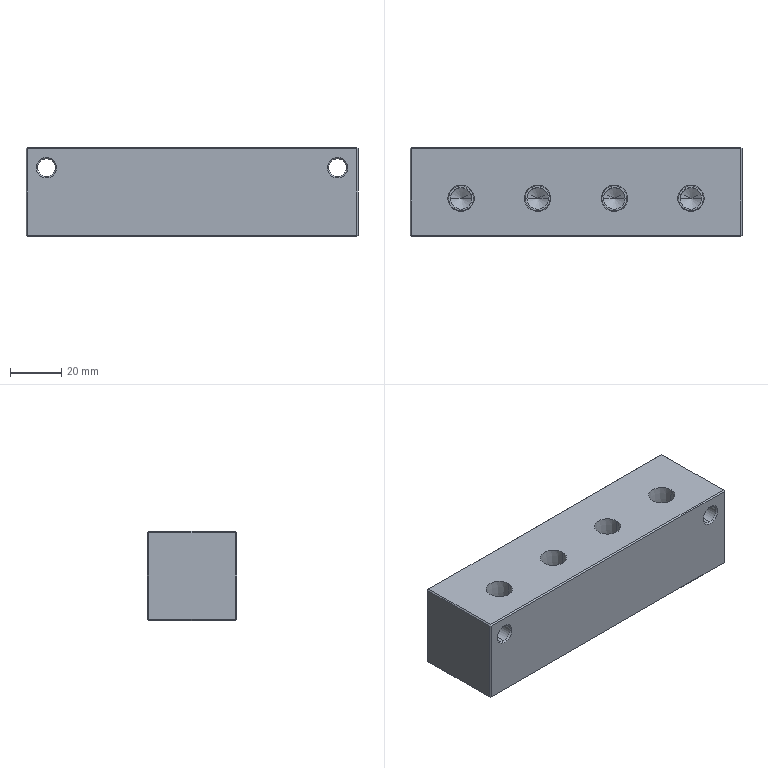Part | STEP file | OP10-012_junction block (C) | 1 solid | 96 faces | box 130 x 35 x 35 mm | volume 144755 mm3 | plane 36 | cone 32 | cylinder 28 | commonest cylinder face diameters 8.433 x20 7 x4 11 x4